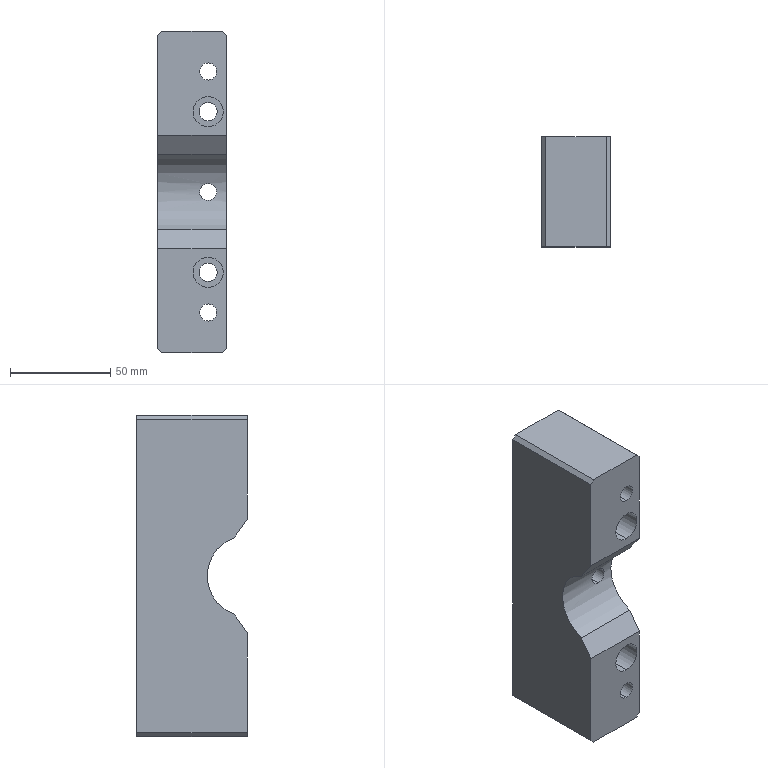Part | SolidWorks | features Chamfer 2, HoleWzd 2, Extrusion 1, ICE 1 | 1 solid | 30 faces | box 34 x 55 x 160 mm | volume 251328 mm3 | cylinder 15 | plane 15 | commonest cylinder face diameters 8.5 x6 9 x4 15 x4 40 x1
STEP:
#1=CARTESIAN_POINT('',(8.,40.,47.5));
#2=VERTEX_POINT('',#1);
#3=CARTESIAN_POINT('',(8.,40.,32.5));
#4=VERTEX_POINT('',#3);
#5=CARTESIAN_POINT('',(8.,40.,40.));
#6=DIRECTION('',(0.,-1.,0.));
#7=DIRECTION('',(0.,0.,-1.));
#8=AXIS2_PLACEMENT_3D('',#5,#6,#7);
#9=CIRCLE('',#8,7.5);
#10=EDGE_CURVE('',#2,#4,#9,.T.);
#11=ORIENTED_EDGE('',*,*,#10,.F.);
#12=CARTESIAN_POINT('',(8.,0.,47.5));
#13=VERTEX_POINT('',#12);
#14=CARTESIAN_POINT('',(8.,0.,47.5));
#15=DIRECTION('',(0.,-1.,0.));
#16=VECTOR('',#15,1000.);
#17=LINE('',#14,#16);
#18=EDGE_CURVE('',#2,#13,#17,.T.);
#19=ORIENTED_EDGE('',*,*,#18,.T.);
#20=CARTESIAN_POINT('',(8.,0.,32.5));
#21=VERTEX_POINT('',#20);
#22=CARTESIAN_POINT('',(8.,0.,40.));
#23=DIRECTION('',(0.,-1.,0.));
#24=DIRECTION('',(0.,0.,-1.));
#25=AXIS2_PLACEMENT_3D('',#22,#23,#24);
#26=CIRCLE('',#25,7.5);
#27=EDGE_CURVE('',#13,#21,#26,.T.);
#28=ORIENTED_EDGE('',*,*,#27,.T.);
#29=CARTESIAN_POINT('',(8.,0.,32.5));
#30=DIRECTION('',(0.,-1.,0.));
#31=VECTOR('',#30,1000.);
#32=LINE('',#29,#31);
#33=EDGE_CURVE('',#4,#21,#32,.T.);
#34=ORIENTED_EDGE('',*,*,#33,.F.);
#35=EDGE_LOOP('',(#11,#19,#28,#34));
#36=FACE_OUTER_BOUND('',#35,.T.);
#37=CARTESIAN_POINT('',(8.,0.,40.));
#38=DIRECTION('',(0.,-1.,0.));
#39=DIRECTION('',(0.,0.,-1.));
#40=AXIS2_PLACEMENT_3D('',#37,#38,#39);
#41=CYLINDRICAL_SURFACE('',#40,7.5);
#42=ADVANCED_FACE('',(#36),#41,.F.);
#43=CARTESIAN_POINT('',(8.,55.,44.5));
#44=VERTEX_POINT('',#43);
#45=CARTESIAN_POINT('',(8.,55.,35.5));
#46=VERTEX_POINT('',#45);
#47=CARTESIAN_POINT('',(8.,55.,40.));
#48=DIRECTION('',(0.,-1.,0.));
#49=DIRECTION('',(0.,0.,-1.));
#50=AXIS2_PLACEMENT_3D('',#47,#48,#49);
#51=CIRCLE('',#50,4.5);
#52=EDGE_CURVE('',#44,#46,#51,.T.);
#53=ORIENTED_EDGE('',*,*,#52,.F.);
#54=CARTESIAN_POINT('',(8.,40.,44.5));
#55=VERTEX_POINT('',#54);
#56=CARTESIAN_POINT('',(8.,0.,44.5));
#57=DIRECTION('',(0.,-1.,0.));
#58=VECTOR('',#57,1000.);
#59=LINE('',#56,#58);
#60=EDGE_CURVE('',#44,#55,#59,.T.);
#61=ORIENTED_EDGE('',*,*,#60,.T.);
#62=CARTESIAN_POINT('',(8.,40.,35.5));
#63=VERTEX_POINT('',#62);
#64=CARTESIAN_POINT('',(8.,40.,40.));
#65=DIRECTION('',(0.,-1.,0.));
#66=DIRECTION('',(0.,0.,-1.));
#67=AXIS2_PLACEMENT_3D('',#64,#65,#66);
#68=CIRCLE('',#67,4.5);
#69=EDGE_CURVE('',#55,#63,#68,.T.);
#70=ORIENTED_EDGE('',*,*,#69,.T.);
#71=CARTESIAN_POINT('',(8.,0.,35.5));
#72=DIRECTION('',(0.,-1.,0.));
#73=VECTOR('',#72,1000.);
#74=LINE('',#71,#73);
#75=EDGE_CURVE('',#46,#63,#74,.T.);
#76=ORIENTED_EDGE('',*,*,#75,.F.);
#77=EDGE_LOOP('',(#53,#61,#70,#76));
#78=FACE_OUTER_BOUND('',#77,.T.);
#79=CARTESIAN_POINT('',(8.,0.,40.));
#80=DIRECTION('',(0.,-1.,0.));
#81=DIRECTION('',(0.,0.,-1.));
#82=AXIS2_PLACEMENT_3D('',#79,#80,#81);
#83=CYLINDRICAL_SURFACE('',#82,4.5);
#84=ADVANCED_FACE('',(#78),#83,.F.);
#85=CARTESIAN_POINT('',(8.,40.,-32.5));
#86=VERTEX_POINT('',#85);
#87=CARTESIAN_POINT('',(8.,40.,-47.5));
#88=VERTEX_POINT('',#87);
#89=CARTESIAN_POINT('',(8.,40.,-40.));
#90=DIRECTION('',(0.,-1.,0.));
#91=DIRECTION('',(0.,0.,-1.));
#92=AXIS2_PLACEMENT_3D('',#89,#90,#91);
#93=CIRCLE('',#92,7.5);
#94=EDGE_CURVE('',#86,#88,#93,.T.);
#95=ORIENTED_EDGE('',*,*,#94,.F.);
#96=CARTESIAN_POINT('',(8.,0.,-32.5));
#97=VERTEX_POINT('',#96);
#98=CARTESIAN_POINT('',(8.,0.,-32.5));
#99=DIRECTION('',(0.,-1.,0.));
#100=VECTOR('',#99,1000.);
#101=LINE('',#98,#100);
#102=EDGE_CURVE('',#86,#97,#101,.T.);
#103=ORIENTED_EDGE('',*,*,#102,.T.);
#104=CARTESIAN_POINT('',(8.,0.,-47.5));
#105=VERTEX_POINT('',#104);
#106=CARTESIAN_POINT('',(8.,0.,-40.));
#107=DIRECTION('',(0.,-1.,0.));
#108=DIRECTION('',(0.,0.,-1.));
#109=AXIS2_PLACEMENT_3D('',#106,#107,#108);
#110=CIRCLE('',#109,7.5);
#111=EDGE_CURVE('',#97,#105,#110,.T.);
#112=ORIENTED_EDGE('',*,*,#111,.T.);
#113=CARTESIAN_POINT('',(8.,0.,-47.5));
#114=DIRECTION('',(0.,-1.,0.));
#115=VECTOR('',#114,1000.);
#116=LINE('',#113,#115);
#117=EDGE_CURVE('',#88,#105,#116,.T.);
#118=ORIENTED_EDGE('',*,*,#117,.F.);
#119=EDGE_LOOP('',(#95,#103,#112,#118));
#120=FACE_OUTER_BOUND('',#119,.T.);
#121=CARTESIAN_POINT('',(8.,0.,-40.));
#122=DIRECTION('',(0.,-1.,0.));
#123=DIRECTION('',(0.,0.,-1.));
#124=AXIS2_PLACEMENT_3D('',#121,#122,#123);
#125=CYLINDRICAL_SURFACE('',#124,7.5);
#126=ADVANCED_FACE('',(#120),#125,.F.);
#127=CARTESIAN_POINT('',(8.,55.,-35.5));
#128=VERTEX_POINT('',#127);
#129=CARTESIAN_POINT('',(8.,55.,-44.5));
#130=VERTEX_POINT('',#129);
#131=CARTESIAN_POINT('',(8.,55.,-40.));
#132=DIRECTION('',(0.,-1.,0.));
#133=DIRECTION('',(0.,0.,-1.));
#134=AXIS2_PLACEMENT_3D('',#131,#132,#133);
#135=CIRCLE('',#134,4.5);
#136=EDGE_CURVE('',#128,#130,#135,.T.);
#137=ORIENTED_EDGE('',*,*,#136,.F.);
#138=CARTESIAN_POINT('',(8.,40.,-35.5));
#139=VERTEX_POINT('',#138);
#140=CARTESIAN_POINT('',(8.,0.,-35.5));
#141=DIRECTION('',(0.,-1.,0.));
#142=VECTOR('',#141,1000.);
#143=LINE('',#140,#142);
#144=EDGE_CURVE('',#128,#139,#143,.T.);
#145=ORIENTED_EDGE('',*,*,#144,.T.);
#146=CARTESIAN_POINT('',(8.,40.,-44.5));
#147=VERTEX_POINT('',#146);
#148=CARTESIAN_POINT('',(8.,40.,-40.));
#149=DIRECTION('',(0.,-1.,0.));
#150=DIRECTION('',(0.,0.,-1.));
#151=AXIS2_PLACEMENT_3D('',#148,#149,#150);
#152=CIRCLE('',#151,4.5);
#153=EDGE_CURVE('',#139,#147,#152,.T.);
#154=ORIENTED_EDGE('',*,*,#153,.T.);
#155=CARTESIAN_POINT('',(8.,0.,-44.5));
#156=DIRECTION('',(0.,-1.,0.));
#157=VECTOR('',#156,1000.);
#158=LINE('',#155,#157);
#159=EDGE_CURVE('',#130,#147,#158,.T.);
#160=ORIENTED_EDGE('',*,*,#159,.F.);
#161=EDGE_LOOP('',(#137,#145,#154,#160));
#162=FACE_OUTER_BOUND('',#161,.T.);
#163=CARTESIAN_POINT('',(8.,0.,-40.));
#164=DIRECTION('',(0.,-1.,0.));
#165=DIRECTION('',(0.,0.,-1.));
#166=AXIS2_PLACEMENT_3D('',#163,#164,#165);
#167=CYLINDRICAL_SURFACE('',#166,4.5);
#168=ADVANCED_FACE('',(#162),#167,.F.);
#169=CARTESIAN_POINT('',(8.,0.,-64.25));
#170=VERTEX_POINT('',#169);
#171=CARTESIAN_POINT('',(8.,0.,-55.75));
#172=VERTEX_POINT('',#171);
#173=CARTESIAN_POINT('',(8.,0.,-60.));
#174=DIRECTION('',(0.,1.,0.));
#175=DIRECTION('',(0.,0.,1.));
#176=AXIS2_PLACEMENT_3D('',#173,#174,#175);
#177=CIRCLE('',#176,4.25);
#178=EDGE_CURVE('',#170,#172,#177,.T.);
#179=ORIENTED_EDGE('',*,*,#178,.F.);
#180=CARTESIAN_POINT('',(8.,55.,-64.25));
#181=VERTEX_POINT('',#180);
#182=CARTESIAN_POINT('',(8.,55.,-64.25));
#183=DIRECTION('',(0.,1.,0.));
#184=VECTOR('',#183,1000.);
#185=LINE('',#182,#184);
#186=EDGE_CURVE('',#170,#181,#185,.T.);
#187=ORIENTED_EDGE('',*,*,#186,.T.);
#188=CARTESIAN_POINT('',(8.,55.,-55.75));
#189=VERTEX_POINT('',#188);
#190=CARTESIAN_POINT('',(8.,55.,-60.));
#191=DIRECTION('',(0.,1.,0.));
#192=DIRECTION('',(0.,0.,1.));
#193=AXIS2_PLACEMENT_3D('',#190,#191,#192);
#194=CIRCLE('',#193,4.25);
#195=EDGE_CURVE('',#181,#189,#194,.T.);
#196=ORIENTED_EDGE('',*,*,#195,.T.);
#197=CARTESIAN_POINT('',(8.,55.,-55.75));
#198=DIRECTION('',(0.,1.,0.));
#199=VECTOR('',#198,1000.);
#200=LINE('',#197,#199);
#201=EDGE_CURVE('',#172,#189,#200,.T.);
#202=ORIENTED_EDGE('',*,*,#201,.F.);
#203=EDGE_LOOP('',(#179,#187,#196,#202));
#204=FACE_OUTER_BOUND('',#203,.T.);
#205=CARTESIAN_POINT('',(8.,55.,-60.));
#206=DIRECTION('',(0.,1.,0.));
#207=DIRECTION('',(0.,0.,1.));
#208=AXIS2_PLACEMENT_3D('',#205,#206,#207);
#209=CYLINDRICAL_SURFACE('',#208,4.25);
#210=ADVANCED_FACE('',(#204),#209,.F.);
#211=CARTESIAN_POINT('',(8.,19.543,4.25));
#212=VERTEX_POINT('',#211);
#213=CARTESIAN_POINT('',(8.,19.543,-4.25));
#214=VERTEX_POINT('',#213);
#215=CARTESIAN_POINT('',(8.,19.543,4.25));
#216=CARTESIAN_POINT('',(7.718,19.543,4.25));
#217=CARTESIAN_POINT('',(7.442,19.549,4.222));
#218=CARTESIAN_POINT('',(6.897,19.572,4.114));
#219=CARTESIAN_POINT('',(6.627,19.59,4.032));
#220=CARTESIAN_POINT('',(6.113,19.632,3.818));
#221=CARTESIAN_POINT('',(5.869,19.658,3.687));
#222=CARTESIAN_POINT('',(5.407,19.713,3.379));
#223=CARTESIAN_POINT('',(5.19,19.743,3.2));
#224=CARTESIAN_POINT('',(4.799,19.803,2.809));
#225=CARTESIAN_POINT('',(4.623,19.832,2.596));
#226=CARTESIAN_POINT('',(4.312,19.888,2.131));
#227=CARTESIAN_POINT('',(4.181,19.913,1.885));
#228=CARTESIAN_POINT('',(3.969,19.954,1.374));
#229=CARTESIAN_POINT('',(3.887,19.971,1.105));
#230=CARTESIAN_POINT('',(3.777,19.994,0.5561));
#231=CARTESIAN_POINT('',(3.75,20.,0.2798));
#232=CARTESIAN_POINT('',(3.75,20.,-0.2764));
#233=CARTESIAN_POINT('',(3.778,19.994,-0.559));
#234=CARTESIAN_POINT('',(3.887,19.971,-1.105));
#235=CARTESIAN_POINT('',(3.967,19.955,-1.37));
#236=CARTESIAN_POINT('',(4.181,19.913,-1.886));
#237=CARTESIAN_POINT('',(4.314,19.887,-2.133));
#238=CARTESIAN_POINT('',(4.621,19.833,-2.593));
#239=CARTESIAN_POINT('',(4.798,19.803,-2.808));
#240=CARTESIAN_POINT('',(5.193,19.743,-3.203));
#241=CARTESIAN_POINT('',(5.406,19.713,-3.378));
#242=CARTESIAN_POINT('',(5.866,19.658,-3.686));
#243=CARTESIAN_POINT('',(6.115,19.632,-3.819));
#244=CARTESIAN_POINT('',(6.629,19.59,-4.032));
#245=CARTESIAN_POINT('',(6.894,19.573,-4.113));
#246=CARTESIAN_POINT('',(7.44,19.549,-4.222));
#247=CARTESIAN_POINT('',(7.722,19.543,-4.25));
#248=CARTESIAN_POINT('',(8.,19.543,-4.25));
#249=B_SPLINE_CURVE_WITH_KNOTS('',3,(#215,#216,#217,#218,#219,#220,#221,#222,#223,#224,#225,#226,#227,#228,#229,#230,#231,#232,#233,#234,#235,#236,#237,#238,#239,#240,#241,#242,#243,#244,#245,#246,#247,#248),.UNSPECIFIED.,.F.,.F.,(4,2,2,2,2,2,2,2,2,2,2,2,2,2,2,2,4),(0.,0.0008328,0.001666,0.002499,0.003331,0.004164,0.004997,0.00583,0.006663,0.007496,0.008328,0.009161,0.009994,0.01083,0.01166,0.01249,0.01333),.UNSPECIFIED.);
#250=EDGE_CURVE('',#212,#214,#249,.T.);
#251=ORIENTED_EDGE('',*,*,#250,.T.);
#252=CARTESIAN_POINT('',(8.,55.,-4.25));
#253=VERTEX_POINT('',#252);
#254=CARTESIAN_POINT('',(8.,55.,-4.25));
#255=DIRECTION('',(0.,1.,0.));
#256=VECTOR('',#255,1000.);
#257=LINE('',#254,#256);
#258=EDGE_CURVE('',#214,#253,#257,.T.);
#259=ORIENTED_EDGE('',*,*,#258,.T.);
#260=CARTESIAN_POINT('',(8.,55.,4.25));
#261=VERTEX_POINT('',#260);
#262=CARTESIAN_POINT('',(8.,55.,0.));
#263=DIRECTION('',(0.,1.,0.));
#264=DIRECTION('',(0.,0.,1.));
#265=AXIS2_PLACEMENT_3D('',#262,#263,#264);
#266=CIRCLE('',#265,4.25);
#267=EDGE_CURVE('',#253,#261,#266,.T.);
#268=ORIENTED_EDGE('',*,*,#267,.T.);
#269=CARTESIAN_POINT('',(8.,55.,4.25));
#270=DIRECTION('',(0.,1.,0.));
#271=VECTOR('',#270,1000.);
#272=LINE('',#269,#271);
#273=EDGE_CURVE('',#212,#261,#272,.T.);
#274=ORIENTED_EDGE('',*,*,#273,.F.);
#275=EDGE_LOOP('',(#251,#259,#268,#274));
#276=FACE_OUTER_BOUND('',#275,.T.);
#277=CARTESIAN_POINT('',(8.,55.,0.));
#278=DIRECTION('',(0.,1.,0.));
#279=DIRECTION('',(0.,0.,1.));
#280=AXIS2_PLACEMENT_3D('',#277,#278,#279);
#281=CYLINDRICAL_SURFACE('',#280,4.25);
#282=ADVANCED_FACE('',(#276),#281,.F.);
#283=CARTESIAN_POINT('',(8.,0.,55.75));
#284=VERTEX_POINT('',#283);
#285=CARTESIAN_POINT('',(8.,0.,64.25));
#286=VERTEX_POINT('',#285);
#287=CARTESIAN_POINT('',(8.,0.,60.));
#288=DIRECTION('',(0.,1.,0.));
#289=DIRECTION('',(0.,0.,1.));
#290=AXIS2_PLACEMENT_3D('',#287,#288,#289);
#291=CIRCLE('',#290,4.25);
#292=EDGE_CURVE('',#284,#286,#291,.T.);
#293=ORIENTED_EDGE('',*,*,#292,.F.);
#294=CARTESIAN_POINT('',(8.,55.,55.75));
#295=VERTEX_POINT('',#294);
#296=CARTESIAN_POINT('',(8.,55.,55.75));
#297=DIRECTION('',(0.,1.,0.));
#298=VECTOR('',#297,1000.);
#299=LINE('',#296,#298);
#300=EDGE_CURVE('',#284,#295,#299,.T.);
#301=ORIENTED_EDGE('',*,*,#300,.T.);
#302=CARTESIAN_POINT('',(8.,55.,64.25));
#303=VERTEX_POINT('',#302);
#304=CARTESIAN_POINT('',(8.,55.,60.));
#305=DIRECTION('',(0.,1.,0.));
#306=DIRECTION('',(0.,0.,1.));
#307=AXIS2_PLACEMENT_3D('',#304,#305,#306);
#308=CIRCLE('',#307,4.25);
#309=EDGE_CURVE('',#295,#303,#308,.T.);
#310=ORIENTED_EDGE('',*,*,#309,.T.);
#311=CARTESIAN_POINT('',(8.,55.,64.25));
#312=DIRECTION('',(0.,1.,0.));
#313=VECTOR('',#312,1000.);
#314=LINE('',#311,#313);
#315=EDGE_CURVE('',#286,#303,#314,.T.);
#316=ORIENTED_EDGE('',*,*,#315,.F.);
#317=EDGE_LOOP('',(#293,#301,#310,#316));
#318=FACE_OUTER_BOUND('',#317,.T.);
#319=CARTESIAN_POINT('',(8.,55.,60.));
#320=DIRECTION('',(0.,1.,0.));
#321=DIRECTION('',(0.,0.,1.));
#322=AXIS2_PLACEMENT_3D('',#319,#320,#321);
#323=CYLINDRICAL_SURFACE('',#322,4.25);
#324=ADVANCED_FACE('',(#318),#323,.F.);
#325=CARTESIAN_POINT('',(8.,0.,60.));
#326=DIRECTION('',(0.,1.,0.));
#327=DIRECTION('',(0.,0.,1.));
#328=AXIS2_PLACEMENT_3D('',#325,#326,#327);
#329=CIRCLE('',#328,4.25);
#330=EDGE_CURVE('',#286,#284,#329,.T.);
#331=ORIENTED_EDGE('',*,*,#330,.T.);
#332=ORIENTED_EDGE('',*,*,#292,.T.);
#333=EDGE_LOOP('',(#331,#332));
#334=FACE_BOUND('',#333,.T.);
#335=CARTESIAN_POINT('',(8.,0.,40.));
#336=DIRECTION('',(0.,-1.,0.));
#337=DIRECTION('',(0.,0.,-1.));
#338=AXIS2_PLACEMENT_3D('',#335,#336,#337);
#339=CIRCLE('',#338,7.5);
#340=EDGE_CURVE('',#21,#13,#339,.T.);
#341=ORIENTED_EDGE('',*,*,#340,.F.);
#342=ORIENTED_EDGE('',*,*,#27,.F.);
#343=EDGE_LOOP('',(#341,#342));
#344=FACE_BOUND('',#343,.T.);
#345=CARTESIAN_POINT('',(-17.,0.,28.284));
#346=VERTEX_POINT('',#345);
#347=CARTESIAN_POINT('',(-17.,0.,78.));
#348=VERTEX_POINT('',#347);
#349=CARTESIAN_POINT('',(-17.,0.,-80.));
#350=DIRECTION('',(0.,0.,1.));
#351=VECTOR('',#350,1000.);
#352=LINE('',#349,#351);
#353=EDGE_CURVE('',#346,#348,#352,.T.);
#354=ORIENTED_EDGE('',*,*,#353,.F.);
#355=CARTESIAN_POINT('',(17.,0.,28.284));
#356=VERTEX_POINT('',#355);
#357=CARTESIAN_POINT('',(0.,0.,28.284));
#358=DIRECTION('',(1.,0.,0.));
#359=VECTOR('',#358,1000.);
#360=LINE('',#357,#359);
#361=EDGE_CURVE('',#346,#356,#360,.T.);
#362=ORIENTED_EDGE('',*,*,#361,.T.);
#363=CARTESIAN_POINT('',(17.,0.,78.));
#364=VERTEX_POINT('',#363);
#365=CARTESIAN_POINT('',(17.,0.,-80.));
#366=DIRECTION('',(0.,0.,-1.));
#367=VECTOR('',#366,1000.);
#368=LINE('',#365,#367);
#369=EDGE_CURVE('',#364,#356,#368,.T.);
#370=ORIENTED_EDGE('',*,*,#369,.F.);
#371=CARTESIAN_POINT('',(15.,0.,80.));
#372=VERTEX_POINT('',#371);
#373=CARTESIAN_POINT('',(17.,0.,78.));
#374=DIRECTION('',(-0.7071,0.,0.7071));
#375=VECTOR('',#374,1000.);
#376=LINE('',#373,#375);
#377=EDGE_CURVE('',#364,#372,#376,.T.);
#378=ORIENTED_EDGE('',*,*,#377,.T.);
#379=CARTESIAN_POINT('',(-15.,0.,80.));
#380=VERTEX_POINT('',#379);
#381=CARTESIAN_POINT('',(-17.,0.,80.));
#382=DIRECTION('',(1.,0.,0.));
#383=VECTOR('',#382,1000.);
#384=LINE('',#381,#383);
#385=EDGE_CURVE('',#380,#372,#384,.T.);
#386=ORIENTED_EDGE('',*,*,#385,.F.);
#387=CARTESIAN_POINT('',(-15.,0.,80.));
#388=DIRECTION('',(-0.7071,0.,-0.7071));
#389=VECTOR('',#388,1000.);
#390=LINE('',#387,#389);
#391=EDGE_CURVE('',#380,#348,#390,.T.);
#392=ORIENTED_EDGE('',*,*,#391,.T.);
#393=EDGE_LOOP('',(#354,#362,#370,#378,#386,#392));
#394=FACE_OUTER_BOUND('',#393,.T.);
#395=CARTESIAN_POINT('',(0.,0.,0.));
#396=DIRECTION('',(0.,1.,0.));
#397=DIRECTION('',(0.,0.,1.));
#398=AXIS2_PLACEMENT_3D('',#395,#396,#397);
#399=PLANE('',#398);
#400=ADVANCED_FACE('',(#334,#344,#394),#399,.F.);
#401=CARTESIAN_POINT('',(17.,6.667,-18.856));
#402=VERTEX_POINT('',#401);
#403=CARTESIAN_POINT('',(17.,6.667,18.856));
#404=VERTEX_POINT('',#403);
#405=CARTESIAN_POINT('',(17.,0.,0.));
#406=DIRECTION('',(1.,0.,0.));
#407=DIRECTION('',(0.,0.,-1.));
#408=AXIS2_PLACEMENT_3D('',#405,#406,#407);
#409=CIRCLE('',#408,20.);
#410=EDGE_CURVE('',#402,#404,#409,.T.);
#411=ORIENTED_EDGE('',*,*,#410,.F.);
#412=CARTESIAN_POINT('',(17.,0.,-28.284));
#413=VERTEX_POINT('',#412);
#414=CARTESIAN_POINT('',(17.,0.,-28.284));
#415=DIRECTION('',(0.,-0.5774,-0.8165));
#416=VECTOR('',#415,1000.);
#417=LINE('',#414,#416);
#418=EDGE_CURVE('',#402,#413,#417,.T.);
#419=ORIENTED_EDGE('',*,*,#418,.T.);
#420=CARTESIAN_POINT('',(17.,0.,-78.));
#421=VERTEX_POINT('',#420);
#422=CARTESIAN_POINT('',(17.,0.,-80.));
#423=DIRECTION('',(0.,0.,-1.));
#424=VECTOR('',#423,1000.);
#425=LINE('',#422,#424);
#426=EDGE_CURVE('',#413,#421,#425,.T.);
#427=ORIENTED_EDGE('',*,*,#426,.T.);
#428=CARTESIAN_POINT('',(17.,55.,-78.));
#429=VERTEX_POINT('',#428);
#430=CARTESIAN_POINT('',(17.,55.,-78.));
#431=DIRECTION('',(0.,1.,0.));
#432=VECTOR('',#431,1000.);
#433=LINE('',#430,#432);
#434=EDGE_CURVE('',#421,#429,#433,.T.);
#435=ORIENTED_EDGE('',*,*,#434,.T.);
#436=CARTESIAN_POINT('',(17.,55.,78.));
#437=VERTEX_POINT('',#436);
#438=CARTESIAN_POINT('',(17.,55.,-80.));
#439=DIRECTION('',(0.,0.,-1.));
#440=VECTOR('',#439,1000.);
#441=LINE('',#438,#440);
#442=EDGE_CURVE('',#437,#429,#441,.T.);
#443=ORIENTED_EDGE('',*,*,#442,.F.);
#444=CARTESIAN_POINT('',(17.,55.,78.));
#445=DIRECTION('',(0.,-1.,0.));
#446=VECTOR('',#445,1000.);
#447=LINE('',#444,#446);
#448=EDGE_CURVE('',#437,#364,#447,.T.);
#449=ORIENTED_EDGE('',*,*,#448,.T.);
#450=ORIENTED_EDGE('',*,*,#369,.T.);
#451=CARTESIAN_POINT('',(17.,0.,28.284));
#452=DIRECTION('',(0.,0.5774,-0.8165));
#453=VECTOR('',#452,1000.);
#454=LINE('',#451,#453);
#455=EDGE_CURVE('',#356,#404,#454,.T.);
#456=ORIENTED_EDGE('',*,*,#455,.T.);
#457=EDGE_LOOP('',(#411,#419,#427,#435,#443,#449,#450,#456));
#458=FACE_OUTER_BOUND('',#457,.T.);
#459=CARTESIAN_POINT('',(17.,55.,-80.));
#460=DIRECTION('',(-1.,0.,0.));
#461=DIRECTION('',(0.,0.,1.));
#462=AXIS2_PLACEMENT_3D('',#459,#460,#461);
#463=PLANE('',#462);
#464=ADVANCED_FACE('',(#458),#463,.F.);
#465=CARTESIAN_POINT('',(15.,55.,-80.));
#466=VERTEX_POINT('',#465);
#467=CARTESIAN_POINT('',(-15.,55.,-80.));
#468=VERTEX_POINT('',#467);
#469=CARTESIAN_POINT('',(-17.,55.,-80.));
#470=DIRECTION('',(-1.,0.,0.));
#471=VECTOR('',#470,1000.);
#472=LINE('',#469,#471);
#473=EDGE_CURVE('',#466,#468,#472,.T.);
#474=ORIENTED_EDGE('',*,*,#473,.F.);
#475=CARTESIAN_POINT('',(15.,0.,-80.));
#476=VERTEX_POINT('',#475);
#477=CARTESIAN_POINT('',(15.,55.,-80.));
#478=DIRECTION('',(0.,-1.,0.));
#479=VECTOR('',#478,1000.);
#480=LINE('',#477,#479);
#481=EDGE_CURVE('',#466,#476,#480,.T.);
#482=ORIENTED_EDGE('',*,*,#481,.T.);
#483=CARTESIAN_POINT('',(-15.,0.,-80.));
#484=VERTEX_POINT('',#483);
#485=CARTESIAN_POINT('',(-17.,0.,-80.));
#486=DIRECTION('',(-1.,0.,0.));
#487=VECTOR('',#486,1000.);
#488=LINE('',#485,#487);
#489=EDGE_CURVE('',#476,#484,#488,.T.);
#490=ORIENTED_EDGE('',*,*,#489,.T.);
#491=CARTESIAN_POINT('',(-15.,55.,-80.));
#492=DIRECTION('',(0.,1.,0.));
#493=VECTOR('',#492,1000.);
#494=LINE('',#491,#493);
#495=EDGE_CURVE('',#484,#468,#494,.T.);
#496=ORIENTED_EDGE('',*,*,#495,.T.);
#497=EDGE_LOOP('',(#474,#482,#490,#496));
#498=FACE_OUTER_BOUND('',#497,.T.);
#499=CARTESIAN_POINT('',(-17.,55.,-80.));
#500=DIRECTION('',(0.,0.,1.));
#501=DIRECTION('',(1.,0.,0.));
#502=AXIS2_PLACEMENT_3D('',#499,#500,#501);
#503=PLANE('',#502);
#504=ADVANCED_FACE('',(#498),#503,.F.);
#505=CARTESIAN_POINT('',(-17.,0.,-78.));
#506=VERTEX_POINT('',#505);
#507=CARTESIAN_POINT('',(-17.,0.,-28.284));
#508=VERTEX_POINT('',#507);
#509=CARTESIAN_POINT('',(-17.,0.,-80.));
#510=DIRECTION('',(0.,0.,1.));
#511=VECTOR('',#510,1000.);
#512=LINE('',#509,#511);
#513=EDGE_CURVE('',#506,#508,#512,.T.);
#514=ORIENTED_EDGE('',*,*,#513,.T.);
#515=CARTESIAN_POINT('',(-17.,6.667,-18.856));
#516=VERTEX_POINT('',#515);
#517=CARTESIAN_POINT('',(-17.,0.,-28.284));
#518=DIRECTION('',(0.,0.5774,0.8165));
#519=VECTOR('',#518,1000.);
#520=LINE('',#517,#519);
#521=EDGE_CURVE('',#508,#516,#520,.T.);
#522=ORIENTED_EDGE('',*,*,#521,.T.);
#523=CARTESIAN_POINT('',(-17.,6.667,18.856));
#524=VERTEX_POINT('',#523);
#525=CARTESIAN_POINT('',(-17.,0.,0.));
#526=DIRECTION('',(1.,0.,0.));
#527=DIRECTION('',(0.,0.,-1.));
#528=AXIS2_PLACEMENT_3D('',#525,#526,#527);
#529=CIRCLE('',#528,20.);
#530=EDGE_CURVE('',#516,#524,#529,.T.);
#531=ORIENTED_EDGE('',*,*,#530,.T.);
#532=CARTESIAN_POINT('',(-17.,0.,28.284));
#533=DIRECTION('',(0.,-0.5774,0.8165));
#534=VECTOR('',#533,1000.);
#535=LINE('',#532,#534);
#536=EDGE_CURVE('',#524,#346,#535,.T.);
#537=ORIENTED_EDGE('',*,*,#536,.T.);
#538=ORIENTED_EDGE('',*,*,#353,.T.);
#539=CARTESIAN_POINT('',(-17.,55.,78.));
#540=VERTEX_POINT('',#539);
#541=CARTESIAN_POINT('',(-17.,55.,78.));
#542=DIRECTION('',(0.,1.,0.));
#543=VECTOR('',#542,1000.);
#544=LINE('',#541,#543);
#545=EDGE_CURVE('',#348,#540,#544,.T.);
#546=ORIENTED_EDGE('',*,*,#545,.T.);
#547=CARTESIAN_POINT('',(-17.,55.,-78.));
#548=VERTEX_POINT('',#547);
#549=CARTESIAN_POINT('',(-17.,55.,-80.));
#550=DIRECTION('',(0.,0.,1.));
#551=VECTOR('',#550,1000.);
#552=LINE('',#549,#551);
#553=EDGE_CURVE('',#548,#540,#552,.T.);
#554=ORIENTED_EDGE('',*,*,#553,.F.);
#555=CARTESIAN_POINT('',(-17.,55.,-78.));
#556=DIRECTION('',(0.,-1.,0.));
#557=VECTOR('',#556,1000.);
#558=LINE('',#555,#557);
#559=EDGE_CURVE('',#548,#506,#558,.T.);
#560=ORIENTED_EDGE('',*,*,#559,.T.);
#561=EDGE_LOOP('',(#514,#522,#531,#537,#538,#546,#554,#560));
#562=FACE_OUTER_BOUND('',#561,.T.);
#563=CARTESIAN_POINT('',(-17.,55.,-80.));
#564=DIRECTION('',(1.,0.,0.));
#565=DIRECTION('',(0.,0.,-1.));
#566=AXIS2_PLACEMENT_3D('',#563,#564,#565);
#567=PLANE('',#566);
#568=ADVANCED_FACE('',(#562),#567,.F.);
#569=CARTESIAN_POINT('',(-15.,55.,80.));
#570=VERTEX_POINT('',#569);
#571=CARTESIAN_POINT('',(15.,55.,80.));
#572=VERTEX_POINT('',#571);
#573=CARTESIAN_POINT('',(-17.,55.,80.));
#574=DIRECTION('',(1.,0.,0.));
#575=VECTOR('',#574,1000.);
#576=LINE('',#573,#575);
#577=EDGE_CURVE('',#570,#572,#576,.T.);
#578=ORIENTED_EDGE('',*,*,#577,.F.);
#579=CARTESIAN_POINT('',(-15.,55.,80.));
#580=DIRECTION('',(0.,-1.,0.));
#581=VECTOR('',#580,1000.);
#582=LINE('',#579,#581);
#583=EDGE_CURVE('',#570,#380,#582,.T.);
#584=ORIENTED_EDGE('',*,*,#583,.T.);
#585=ORIENTED_EDGE('',*,*,#385,.T.);
#586=CARTESIAN_POINT('',(15.,55.,80.));
#587=DIRECTION('',(0.,1.,0.));
#588=VECTOR('',#587,1000.);
#589=LINE('',#586,#588);
#590=EDGE_CURVE('',#372,#572,#589,.T.);
#591=ORIENTED_EDGE('',*,*,#590,.T.);
#592=EDGE_LOOP('',(#578,#584,#585,#591));
#593=FACE_OUTER_BOUND('',#592,.T.);
#594=CARTESIAN_POINT('',(-17.,55.,80.));
#595=DIRECTION('',(0.,0.,-1.));
#596=DIRECTION('',(-1.,0.,0.));
#597=AXIS2_PLACEMENT_3D('',#594,#595,#596);
#598=PLANE('',#597);
#599=ADVANCED_FACE('',(#593),#598,.F.);
#600=CARTESIAN_POINT('',(8.,55.,40.));
#601=DIRECTION('',(0.,-1.,0.));
#602=DIRECTION('',(0.,0.,-1.));
#603=AXIS2_PLACEMENT_3D('',#600,#601,#602);
#604=CIRCLE('',#603,4.5);
#605=EDGE_CURVE('',#46,#44,#604,.T.);
#606=ORIENTED_EDGE('',*,*,#605,.T.);
#607=ORIENTED_EDGE('',*,*,#52,.T.);
#608=EDGE_LOOP('',(#606,#607));
#609=FACE_BOUND('',#608,.T.);
#610=CARTESIAN_POINT('',(8.,55.,-40.));
#611=DIRECTION('',(0.,-1.,0.));
#612=DIRECTION('',(0.,0.,-1.));
#613=AXIS2_PLACEMENT_3D('',#610,#611,#612);
#614=CIRCLE('',#613,4.5);
#615=EDGE_CURVE('',#130,#128,#614,.T.);
#616=ORIENTED_EDGE('',*,*,#615,.T.);
#617=ORIENTED_EDGE('',*,*,#136,.T.);
#618=EDGE_LOOP('',(#616,#617));
#619=FACE_BOUND('',#618,.T.);
#620=CARTESIAN_POINT('',(8.,55.,-60.));
#621=DIRECTION('',(0.,1.,0.));
#622=DIRECTION('',(0.,0.,1.));
#623=AXIS2_PLACEMENT_3D('',#620,#621,#622);
#624=CIRCLE('',#623,4.25);
#625=EDGE_CURVE('',#189,#181,#624,.T.);
#626=ORIENTED_EDGE('',*,*,#625,.F.);
#627=ORIENTED_EDGE('',*,*,#195,.F.);
#628=EDGE_LOOP('',(#626,#627));
#629=FACE_BOUND('',#628,.T.);
#630=CARTESIAN_POINT('',(8.,55.,0.));
#631=DIRECTION('',(0.,1.,0.));
#632=DIRECTION('',(0.,0.,1.));
#633=AXIS2_PLACEMENT_3D('',#630,#631,#632);
#634=CIRCLE('',#633,4.25);
#635=EDGE_CURVE('',#261,#253,#634,.T.);
#636=ORIENTED_EDGE('',*,*,#635,.F.);
#637=ORIENTED_EDGE('',*,*,#267,.F.);
#638=EDGE_LOOP('',(#636,#637));
#639=FACE_BOUND('',#638,.T.);
#640=CARTESIAN_POINT('',(8.,55.,60.));
#641=DIRECTION('',(0.,1.,0.));
#642=DIRECTION('',(0.,0.,1.));
#643=AXIS2_PLACEMENT_3D('',#640,#641,#642);
#644=CIRCLE('',#643,4.25);
#645=EDGE_CURVE('',#303,#295,#644,.T.);
#646=ORIENTED_EDGE('',*,*,#645,.F.);
#647=ORIENTED_EDGE('',*,*,#309,.F.);
#648=EDGE_LOOP('',(#646,#647));
#649=FACE_BOUND('',#648,.T.);
#650=ORIENTED_EDGE('',*,*,#553,.T.);
#651=CARTESIAN_POINT('',(-47.5,55.,47.5));
#652=DIRECTION('',(0.7071,0.,0.7071));
#653=VECTOR('',#652,1000.);
#654=LINE('',#651,#653);
#655=EDGE_CURVE('',#540,#570,#654,.T.);
#656=ORIENTED_EDGE('',*,*,#655,.T.);
#657=ORIENTED_EDGE('',*,*,#577,.T.);
#658=CARTESIAN_POINT('',(47.5,55.,47.5));
#659=DIRECTION('',(0.7071,0.,-0.7071));
#660=VECTOR('',#659,1000.);
#661=LINE('',#658,#660);
#662=EDGE_CURVE('',#572,#437,#661,.T.);
#663=ORIENTED_EDGE('',*,*,#662,.T.);
#664=ORIENTED_EDGE('',*,*,#442,.T.);
#665=CARTESIAN_POINT('',(47.5,55.,-47.5));
#666=DIRECTION('',(-0.7071,0.,-0.7071));
#667=VECTOR('',#666,1000.);
#668=LINE('',#665,#667);
#669=EDGE_CURVE('',#429,#466,#668,.T.);
#670=ORIENTED_EDGE('',*,*,#669,.T.);
#671=ORIENTED_EDGE('',*,*,#473,.T.);
#672=CARTESIAN_POINT('',(-47.5,55.,-47.5));
#673=DIRECTION('',(-0.7071,0.,0.7071));
#674=VECTOR('',#673,1000.);
#675=LINE('',#672,#674);
#676=EDGE_CURVE('',#468,#548,#675,.T.);
#677=ORIENTED_EDGE('',*,*,#676,.T.);
#678=EDGE_LOOP('',(#650,#656,#657,#663,#664,#670,#671,#677));
#679=FACE_OUTER_BOUND('',#678,.T.);
#680=CARTESIAN_POINT('',(0.,55.,0.));
#681=DIRECTION('',(0.,1.,0.));
#682=DIRECTION('',(0.,0.,1.));
#683=AXIS2_PLACEMENT_3D('',#680,#681,#682);
#684=PLANE('',#683);
#685=ADVANCED_FACE('',(#609,#619,#629,#639,#649,#679),#684,.T.);
#686=CARTESIAN_POINT('',(8.,0.,-40.));
#687=DIRECTION('',(0.,-1.,0.));
#688=DIRECTION('',(0.,0.,-1.));
#689=AXIS2_PLACEMENT_3D('',#686,#687,#688);
#690=CIRCLE('',#689,7.5);
#691=EDGE_CURVE('',#105,#97,#690,.T.);
#692=ORIENTED_EDGE('',*,*,#691,.F.);
#693=ORIENTED_EDGE('',*,*,#111,.F.);
#694=EDGE_LOOP('',(#692,#693));
#695=FACE_BOUND('',#694,.T.);
#696=CARTESIAN_POINT('',(8.,0.,-60.));
#697=DIRECTION('',(0.,1.,0.));
#698=DIRECTION('',(0.,0.,1.));
#699=AXIS2_PLACEMENT_3D('',#696,#697,#698);
#700=CIRCLE('',#699,4.25);
#701=EDGE_CURVE('',#172,#170,#700,.T.);
#702=ORIENTED_EDGE('',*,*,#701,.T.);
#703=ORIENTED_EDGE('',*,*,#178,.T.);
#704=EDGE_LOOP('',(#702,#703));
#705=FACE_BOUND('',#704,.T.);
#706=ORIENTED_EDGE('',*,*,#426,.F.);
#707=CARTESIAN_POINT('',(0.,0.,-28.284));
#708=DIRECTION('',(-1.,0.,0.));
#709=VECTOR('',#708,1000.);
#710=LINE('',#707,#709);
#711=EDGE_CURVE('',#413,#508,#710,.T.);
#712=ORIENTED_EDGE('',*,*,#711,.T.);
#713=ORIENTED_EDGE('',*,*,#513,.F.);
#714=CARTESIAN_POINT('',(-17.,0.,-78.));
#715=DIRECTION('',(0.7071,0.,-0.7071));
#716=VECTOR('',#715,1000.);
#717=LINE('',#714,#716);
#718=EDGE_CURVE('',#506,#484,#717,.T.);
#719=ORIENTED_EDGE('',*,*,#718,.T.);
#720=ORIENTED_EDGE('',*,*,#489,.F.);
#721=CARTESIAN_POINT('',(15.,0.,-80.));
#722=DIRECTION('',(0.7071,0.,0.7071));
#723=VECTOR('',#722,1000.);
#724=LINE('',#721,#723);
#725=EDGE_CURVE('',#476,#421,#724,.T.);
#726=ORIENTED_EDGE('',*,*,#725,.T.);
#727=EDGE_LOOP('',(#706,#712,#713,#719,#720,#726));
#728=FACE_OUTER_BOUND('',#727,.T.);
#729=CARTESIAN_POINT('',(0.,0.,0.));
#730=DIRECTION('',(0.,1.,0.));
#731=DIRECTION('',(0.,0.,1.));
#732=AXIS2_PLACEMENT_3D('',#729,#730,#731);
#733=PLANE('',#732);
#734=ADVANCED_FACE('',(#695,#705,#728),#733,.F.);
#735=ORIENTED_EDGE('',*,*,#300,.F.);
#736=ORIENTED_EDGE('',*,*,#330,.F.);
#737=ORIENTED_EDGE('',*,*,#315,.T.);
#738=ORIENTED_EDGE('',*,*,#645,.T.);
#739=EDGE_LOOP('',(#735,#736,#737,#738));
#740=FACE_OUTER_BOUND('',#739,.T.);
#741=CARTESIAN_POINT('',(8.,55.,60.));
#742=DIRECTION('',(0.,1.,0.));
#743=DIRECTION('',(0.,0.,1.));
#744=AXIS2_PLACEMENT_3D('',#741,#742,#743);
#745=CYLINDRICAL_SURFACE('',#744,4.25);
#746=ADVANCED_FACE('',(#740),#745,.F.);
#747=ORIENTED_EDGE('',*,*,#258,.F.);
#748=CARTESIAN_POINT('',(8.,19.543,-4.25));
#749=CARTESIAN_POINT('',(8.278,19.543,-4.25));
#750=CARTESIAN_POINT('',(8.554,19.549,-4.223));
#751=CARTESIAN_POINT('',(9.105,19.573,-4.113));
#752=CARTESIAN_POINT('',(9.372,19.59,-4.032));
#753=CARTESIAN_POINT('',(9.884,19.632,-3.82));
#754=CARTESIAN_POINT('',(10.132,19.658,-3.687));
#755=CARTESIAN_POINT('',(10.594,19.713,-3.378));
#756=CARTESIAN_POINT('',(10.807,19.743,-3.203));
#757=CARTESIAN_POINT('',(11.199,19.802,-2.811));
#758=CARTESIAN_POINT('',(11.378,19.833,-2.593));
#759=CARTESIAN_POINT('',(11.686,19.887,-2.133));
#760=CARTESIAN_POINT('',(11.817,19.912,-1.89));
#761=CARTESIAN_POINT('',(12.032,19.954,-1.374));
#762=CARTESIAN_POINT('',(12.113,19.971,-1.105));
#763=CARTESIAN_POINT('',(12.222,19.994,-0.5616));
#764=CARTESIAN_POINT('',(12.25,20.,-0.2824));
#765=CARTESIAN_POINT('',(12.25,20.,0.2786));
#766=CARTESIAN_POINT('',(12.223,19.994,0.555));
#767=CARTESIAN_POINT('',(12.115,19.972,1.1));
#768=CARTESIAN_POINT('',(12.032,19.955,1.371));
#769=CARTESIAN_POINT('',(11.82,19.913,1.884));
#770=CARTESIAN_POINT('',(11.689,19.888,2.128));
#771=CARTESIAN_POINT('',(11.38,19.833,2.591));
#772=CARTESIAN_POINT('',(11.202,19.803,2.808));
#773=CARTESIAN_POINT('',(10.812,19.744,3.199));
#774=CARTESIAN_POINT('',(10.598,19.714,3.375));
#775=CARTESIAN_POINT('',(10.133,19.658,3.687));
#776=CARTESIAN_POINT('',(9.889,19.633,3.817));
#777=CARTESIAN_POINT('',(9.378,19.59,4.03));
#778=CARTESIAN_POINT('',(9.108,19.573,4.113));
#779=CARTESIAN_POINT('',(8.559,19.549,4.222));
#780=CARTESIAN_POINT('',(8.282,19.543,4.25));
#781=CARTESIAN_POINT('',(8.,19.543,4.25));
#782=B_SPLINE_CURVE_WITH_KNOTS('',3,(#748,#749,#750,#751,#752,#753,#754,#755,#756,#757,#758,#759,#760,#761,#762,#763,#764,#765,#766,#767,#768,#769,#770,#771,#772,#773,#774,#775,#776,#777,#778,#779,#780,#781),.UNSPECIFIED.,.F.,.F.,(4,2,2,2,2,2,2,2,2,2,2,2,2,2,2,2,4),(0.01333,0.01416,0.01499,0.01582,0.01666,0.01749,0.01832,0.01915,0.01999,0.02082,0.02165,0.02248,0.02332,0.02415,0.02498,0.02581,0.02665),.UNSPECIFIED.);
#783=EDGE_CURVE('',#214,#212,#782,.T.);
#784=ORIENTED_EDGE('',*,*,#783,.T.);
#785=ORIENTED_EDGE('',*,*,#273,.T.);
#786=ORIENTED_EDGE('',*,*,#635,.T.);
#787=EDGE_LOOP('',(#747,#784,#785,#786));
#788=FACE_OUTER_BOUND('',#787,.T.);
#789=CARTESIAN_POINT('',(8.,55.,0.));
#790=DIRECTION('',(0.,1.,0.));
#791=DIRECTION('',(0.,0.,1.));
#792=AXIS2_PLACEMENT_3D('',#789,#790,#791);
#793=CYLINDRICAL_SURFACE('',#792,4.25);
#794=ADVANCED_FACE('',(#788),#793,.F.);
#795=ORIENTED_EDGE('',*,*,#186,.F.);
#796=ORIENTED_EDGE('',*,*,#701,.F.);
#797=ORIENTED_EDGE('',*,*,#201,.T.);
#798=ORIENTED_EDGE('',*,*,#625,.T.);
#799=EDGE_LOOP('',(#795,#796,#797,#798));
#800=FACE_OUTER_BOUND('',#799,.T.);
#801=CARTESIAN_POINT('',(8.,55.,-60.));
#802=DIRECTION('',(0.,1.,0.));
#803=DIRECTION('',(0.,0.,1.));
#804=AXIS2_PLACEMENT_3D('',#801,#802,#803);
#805=CYLINDRICAL_SURFACE('',#804,4.25);
#806=ADVANCED_FACE('',(#800),#805,.F.);
#807=ORIENTED_EDGE('',*,*,#655,.F.);
#808=ORIENTED_EDGE('',*,*,#545,.F.);
#809=ORIENTED_EDGE('',*,*,#391,.F.);
#810=ORIENTED_EDGE('',*,*,#583,.F.);
#811=EDGE_LOOP('',(#807,#808,#809,#810));
#812=FACE_OUTER_BOUND('',#811,.T.);
#813=CARTESIAN_POINT('',(-15.,55.,80.));
#814=DIRECTION('',(0.7071,0.,-0.7071));
#815=DIRECTION('',(0.,-1.,0.));
#816=AXIS2_PLACEMENT_3D('',#813,#814,#815);
#817=PLANE('',#816);
#818=ADVANCED_FACE('',(#812),#817,.F.);
#819=ORIENTED_EDGE('',*,*,#662,.F.);
#820=ORIENTED_EDGE('',*,*,#590,.F.);
#821=ORIENTED_EDGE('',*,*,#377,.F.);
#822=ORIENTED_EDGE('',*,*,#448,.F.);
#823=EDGE_LOOP('',(#819,#820,#821,#822));
#824=FACE_OUTER_BOUND('',#823,.T.);
#825=CARTESIAN_POINT('',(17.,55.,78.));
#826=DIRECTION('',(-0.7071,0.,-0.7071));
#827=DIRECTION('',(0.,-1.,0.));
#828=AXIS2_PLACEMENT_3D('',#825,#826,#827);
#829=PLANE('',#828);
#830=ADVANCED_FACE('',(#824),#829,.F.);
#831=ORIENTED_EDGE('',*,*,#669,.F.);
#832=ORIENTED_EDGE('',*,*,#434,.F.);
#833=ORIENTED_EDGE('',*,*,#725,.F.);
#834=ORIENTED_EDGE('',*,*,#481,.F.);
#835=EDGE_LOOP('',(#831,#832,#833,#834));
#836=FACE_OUTER_BOUND('',#835,.T.);
#837=CARTESIAN_POINT('',(15.,55.,-80.));
#838=DIRECTION('',(-0.7071,0.,0.7071));
#839=DIRECTION('',(0.,-1.,0.));
#840=AXIS2_PLACEMENT_3D('',#837,#838,#839);
#841=PLANE('',#840);
#842=ADVANCED_FACE('',(#836),#841,.F.);
#843=ORIENTED_EDGE('',*,*,#676,.F.);
#844=ORIENTED_EDGE('',*,*,#495,.F.);
#845=ORIENTED_EDGE('',*,*,#718,.F.);
#846=ORIENTED_EDGE('',*,*,#559,.F.);
#847=EDGE_LOOP('',(#843,#844,#845,#846));
#848=FACE_OUTER_BOUND('',#847,.T.);
#849=CARTESIAN_POINT('',(-17.,55.,-78.));
#850=DIRECTION('',(0.7071,0.,0.7071));
#851=DIRECTION('',(0.,-1.,0.));
#852=AXIS2_PLACEMENT_3D('',#849,#850,#851);
#853=PLANE('',#852);
#854=ADVANCED_FACE('',(#848),#853,.F.);
#855=ORIENTED_EDGE('',*,*,#144,.F.);
#856=ORIENTED_EDGE('',*,*,#615,.F.);
#857=ORIENTED_EDGE('',*,*,#159,.T.);
#858=CARTESIAN_POINT('',(8.,40.,-40.));
#859=DIRECTION('',(0.,-1.,0.));
#860=DIRECTION('',(0.,0.,-1.));
#861=AXIS2_PLACEMENT_3D('',#858,#859,#860);
#862=CIRCLE('',#861,4.5);
#863=EDGE_CURVE('',#147,#139,#862,.T.);
#864=ORIENTED_EDGE('',*,*,#863,.T.);
#865=EDGE_LOOP('',(#855,#856,#857,#864));
#866=FACE_OUTER_BOUND('',#865,.T.);
#867=CARTESIAN_POINT('',(8.,0.,-40.));
#868=DIRECTION('',(0.,-1.,0.));
#869=DIRECTION('',(0.,0.,-1.));
#870=AXIS2_PLACEMENT_3D('',#867,#868,#869);
#871=CYLINDRICAL_SURFACE('',#870,4.5);
#872=ADVANCED_FACE('',(#866),#871,.F.);
#873=ORIENTED_EDGE('',*,*,#863,.F.);
#874=ORIENTED_EDGE('',*,*,#153,.F.);
#875=EDGE_LOOP('',(#873,#874));
#876=FACE_BOUND('',#875,.T.);
#877=CARTESIAN_POINT('',(8.,40.,-40.));
#878=DIRECTION('',(0.,-1.,0.));
#879=DIRECTION('',(0.,0.,-1.));
#880=AXIS2_PLACEMENT_3D('',#877,#878,#879);
#881=CIRCLE('',#880,7.5);
#882=EDGE_CURVE('',#88,#86,#881,.T.);
#883=ORIENTED_EDGE('',*,*,#882,.T.);
#884=ORIENTED_EDGE('',*,*,#94,.T.);
#885=EDGE_LOOP('',(#883,#884));
#886=FACE_OUTER_BOUND('',#885,.T.);
#887=CARTESIAN_POINT('',(12.5,40.,-40.));
#888=DIRECTION('',(0.,1.,0.));
#889=DIRECTION('',(0.,0.,1.));
#890=AXIS2_PLACEMENT_3D('',#887,#888,#889);
#891=PLANE('',#890);
#892=ADVANCED_FACE('',(#876,#886),#891,.F.);
#893=ORIENTED_EDGE('',*,*,#102,.F.);
#894=ORIENTED_EDGE('',*,*,#882,.F.);
#895=ORIENTED_EDGE('',*,*,#117,.T.);
#896=ORIENTED_EDGE('',*,*,#691,.T.);
#897=EDGE_LOOP('',(#893,#894,#895,#896));
#898=FACE_OUTER_BOUND('',#897,.T.);
#899=CARTESIAN_POINT('',(8.,0.,-40.));
#900=DIRECTION('',(0.,-1.,0.));
#901=DIRECTION('',(0.,0.,-1.));
#902=AXIS2_PLACEMENT_3D('',#899,#900,#901);
#903=CYLINDRICAL_SURFACE('',#902,7.5);
#904=ADVANCED_FACE('',(#898),#903,.F.);
#905=ORIENTED_EDGE('',*,*,#60,.F.);
#906=ORIENTED_EDGE('',*,*,#605,.F.);
#907=ORIENTED_EDGE('',*,*,#75,.T.);
#908=CARTESIAN_POINT('',(8.,40.,40.));
#909=DIRECTION('',(0.,-1.,0.));
#910=DIRECTION('',(0.,0.,-1.));
#911=AXIS2_PLACEMENT_3D('',#908,#909,#910);
#912=CIRCLE('',#911,4.5);
#913=EDGE_CURVE('',#63,#55,#912,.T.);
#914=ORIENTED_EDGE('',*,*,#913,.T.);
#915=EDGE_LOOP('',(#905,#906,#907,#914));
#916=FACE_OUTER_BOUND('',#915,.T.);
#917=CARTESIAN_POINT('',(8.,0.,40.));
#918=DIRECTION('',(0.,-1.,0.));
#919=DIRECTION('',(0.,0.,-1.));
#920=AXIS2_PLACEMENT_3D('',#917,#918,#919);
#921=CYLINDRICAL_SURFACE('',#920,4.5);
#922=ADVANCED_FACE('',(#916),#921,.F.);
#923=ORIENTED_EDGE('',*,*,#913,.F.);
#924=ORIENTED_EDGE('',*,*,#69,.F.);
#925=EDGE_LOOP('',(#923,#924));
#926=FACE_BOUND('',#925,.T.);
#927=CARTESIAN_POINT('',(8.,40.,40.));
#928=DIRECTION('',(0.,-1.,0.));
#929=DIRECTION('',(0.,0.,-1.));
#930=AXIS2_PLACEMENT_3D('',#927,#928,#929);
#931=CIRCLE('',#930,7.5);
#932=EDGE_CURVE('',#4,#2,#931,.T.);
#933=ORIENTED_EDGE('',*,*,#932,.T.);
#934=ORIENTED_EDGE('',*,*,#10,.T.);
#935=EDGE_LOOP('',(#933,#934));
#936=FACE_OUTER_BOUND('',#935,.T.);
#937=CARTESIAN_POINT('',(12.5,40.,40.));
#938=DIRECTION('',(0.,1.,0.));
#939=DIRECTION('',(0.,0.,1.));
#940=AXIS2_PLACEMENT_3D('',#937,#938,#939);
#941=PLANE('',#940);
#942=ADVANCED_FACE('',(#926,#936),#941,.F.);
#943=ORIENTED_EDGE('',*,*,#18,.F.);
#944=ORIENTED_EDGE('',*,*,#932,.F.);
#945=ORIENTED_EDGE('',*,*,#33,.T.);
#946=ORIENTED_EDGE('',*,*,#340,.T.);
#947=EDGE_LOOP('',(#943,#944,#945,#946));
#948=FACE_OUTER_BOUND('',#947,.T.);
#949=CARTESIAN_POINT('',(8.,0.,40.));
#950=DIRECTION('',(0.,-1.,0.));
#951=DIRECTION('',(0.,0.,-1.));
#952=AXIS2_PLACEMENT_3D('',#949,#950,#951);
#953=CYLINDRICAL_SURFACE('',#952,7.5);
#954=ADVANCED_FACE('',(#948),#953,.F.);
#955=ORIENTED_EDGE('',*,*,#250,.F.);
#956=ORIENTED_EDGE('',*,*,#783,.F.);
#957=EDGE_LOOP('',(#955,#956));
#958=FACE_BOUND('',#957,.T.);
#959=ORIENTED_EDGE('',*,*,#530,.F.);
#960=CARTESIAN_POINT('',(-17.,6.667,-18.856));
#961=DIRECTION('',(1.,0.,0.));
#962=VECTOR('',#961,1000.);
#963=LINE('',#960,#962);
#964=EDGE_CURVE('',#516,#402,#963,.T.);
#965=ORIENTED_EDGE('',*,*,#964,.T.);
#966=ORIENTED_EDGE('',*,*,#410,.T.);
#967=CARTESIAN_POINT('',(-17.,6.667,18.856));
#968=DIRECTION('',(-1.,0.,0.));
#969=VECTOR('',#968,1000.);
#970=LINE('',#967,#969);
#971=EDGE_CURVE('',#404,#524,#970,.T.);
#972=ORIENTED_EDGE('',*,*,#971,.T.);
#973=EDGE_LOOP('',(#959,#965,#966,#972));
#974=FACE_OUTER_BOUND('',#973,.T.);
#975=CARTESIAN_POINT('',(-17.,0.,0.));
#976=DIRECTION('',(1.,0.,0.));
#977=DIRECTION('',(0.,0.,-1.));
#978=AXIS2_PLACEMENT_3D('',#975,#976,#977);
#979=CYLINDRICAL_SURFACE('',#978,20.);
#980=ADVANCED_FACE('',(#958,#974),#979,.F.);
#981=ORIENTED_EDGE('',*,*,#418,.F.);
#982=ORIENTED_EDGE('',*,*,#964,.F.);
#983=ORIENTED_EDGE('',*,*,#521,.F.);
#984=ORIENTED_EDGE('',*,*,#711,.F.);
#985=EDGE_LOOP('',(#981,#982,#983,#984));
#986=FACE_OUTER_BOUND('',#985,.T.);
#987=CARTESIAN_POINT('',(-17.,0.,-28.284));
#988=DIRECTION('',(0.,-0.8165,0.5774));
#989=DIRECTION('',(1.,0.,0.));
#990=AXIS2_PLACEMENT_3D('',#987,#988,#989);
#991=PLANE('',#990);
#992=ADVANCED_FACE('',(#986),#991,.T.);
#993=ORIENTED_EDGE('',*,*,#536,.F.);
#994=ORIENTED_EDGE('',*,*,#971,.F.);
#995=ORIENTED_EDGE('',*,*,#455,.F.);
#996=ORIENTED_EDGE('',*,*,#361,.F.);
#997=EDGE_LOOP('',(#993,#994,#995,#996));
#998=FACE_OUTER_BOUND('',#997,.T.);
#999=CARTESIAN_POINT('',(-17.,0.,28.284));
#1000=DIRECTION('',(0.,0.8165,0.5774));
#1001=DIRECTION('',(1.,0.,0.));
#1002=AXIS2_PLACEMENT_3D('',#999,#1000,#1001);
#1003=PLANE('',#1002);
#1004=ADVANCED_FACE('',(#998),#1003,.F.);
#1005=CLOSED_SHELL('',(#42,#84,#126,#168,#210,#282,#324,#400,#464,#504,#568,#599,#685,#734,#746,#794,#806,#818,#830,#842,#854,#872,#892,#904,#922,#942,#954,#980,#992,#1004));
#1006=MANIFOLD_SOLID_BREP('',#1005);
#1007=CARTESIAN_POINT('',(0.,0.,0.));
#1008=DIRECTION('',(0.,0.,1.));
#1009=DIRECTION('',(1.,0.,0.));
#1010=AXIS2_PLACEMENT_3D('',#1007,#1008,#1009);
#1011=(LENGTH_UNIT()NAMED_UNIT(*)SI_UNIT(.MILLI.,.METRE.));
#1012=UNCERTAINTY_MEASURE_WITH_UNIT(LENGTH_MEASURE(0.00001),#1011,'','');
#1013=(NAMED_UNIT(*)PLANE_ANGLE_UNIT()SI_UNIT($,.RADIAN.));
#1014=(NAMED_UNIT(*)SI_UNIT($,.STERADIAN.)SOLID_ANGLE_UNIT());
#1015=(GEOMETRIC_REPRESENTATION_CONTEXT(3)GLOBAL_UNCERTAINTY_ASSIGNED_CONTEXT((#1012))GLOBAL_UNIT_ASSIGNED_CONTEXT((#1011,#1013,#1014))REPRESENTATION_CONTEXT('',''));
#1016=ADVANCED_BREP_SHAPE_REPRESENTATION('',(#1006,#1010),#1015);